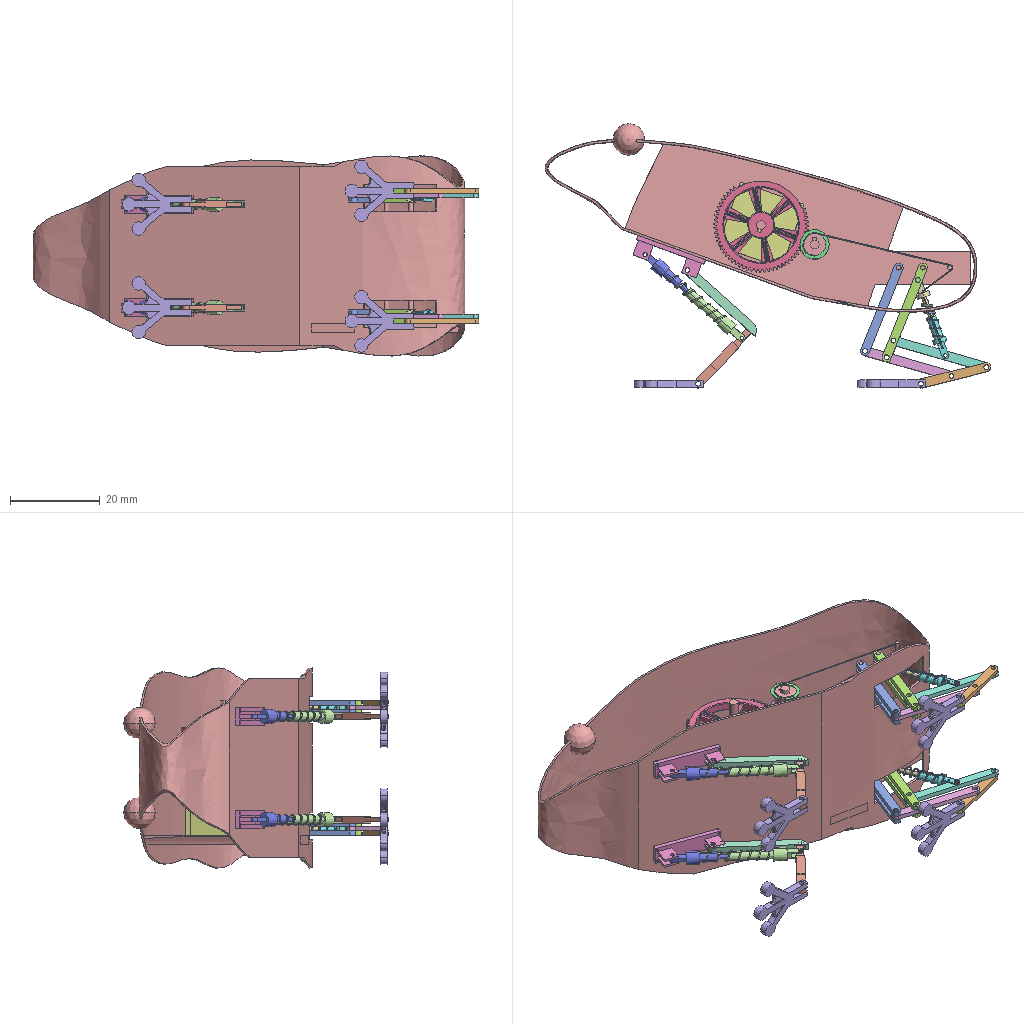Assembly | SolidWorks | 22 different items | 46 placed | box 99 x 59 x 45 mm
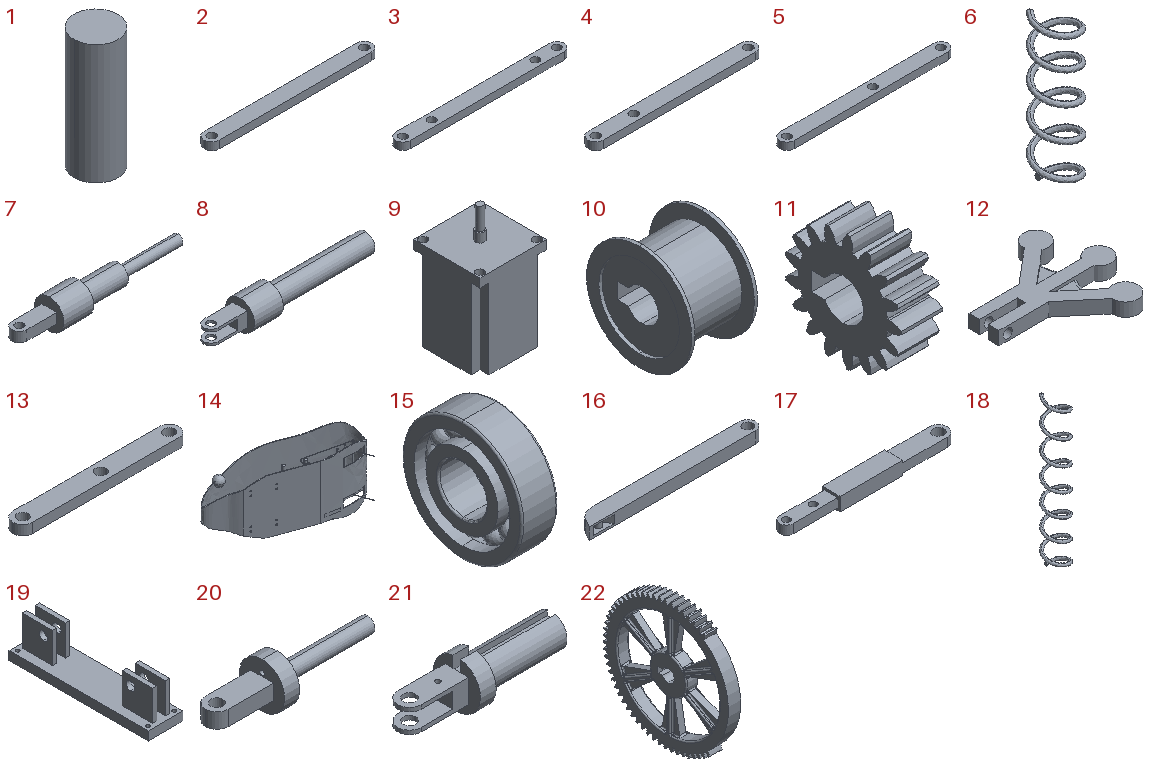Parts list (item | quantity | size | volume | features):
1 | x2 | 1.1 x 1.1 x 3 mm | 2.851 mm3 | features Extrusion 1
2 | x4 | 22 x 2 x 1 mm | 41.241 mm3 | features Extrusion 1, ICE 1
3 | x4 | 23.5 x 2 x 1 mm | 42.34 mm3 | features Extrusion 1, ICE 1
4 | x2 | 22 x 2 x 1 mm | 40.291 mm3 | features Extrusion 1, ICE 1
5 | x2 | 23.5 x 2 x 1 mm | 43.291 mm3 | features Extrusion 1, ICE 1
6 | x2 | 2.421 x 2.42 x 9.051 mm | 2.291 mm3 | features Helix 1, Sweep 1
7 | x2 | 16.75 x 3 x 3 mm | 43.365 mm3 | features ICE 2, Revolution 1
8 | x2 | 16.75 x 3 x 3 mm | 51.85 mm3 | features ICE 3, Revolution 1
9 | x1 | 15 x 15 x 27 mm | 4207 mm3 | features ICE 4, Extrusion 1
10 | x2 | 4.086 x 6.543 x 6.543 mm | 64.18 mm3 | features ICE 1, Revolution 1
11 | x1 | 2 x 5.664 x 5.687 mm | 31.821 mm3 | features BaseBody 1, ICE 1
12 | x4 | 15.281 x 13.766 x 1.6 mm | 106.552 mm3 | features ICE 7, Extrusion 1, Fillet 1, Scale 1
13 | x2 | 17 x 2 x 1 mm | 30.291 mm3 | features Extrusion 1, ICE 1
14 | x1 | 96.052 x 49.979 x 44.528 mm | 8210 mm3 | features ICE 13, MirrorPattern 3, Extrusion 1, Fillet 1, Revolution 1, Sweep 1
15 | x2 | 1.5 x 5 x 5 mm | 18.357 mm3 | features BaseBody 1
16 | x2 | 22.155 x 2 x 1.5 mm | 59.83 mm3 | features Extrusion 1, Fillet 1, ICE 1
17 | x2 | 18.75 x 2 x 1.5 mm | 38.722 mm3 | features ICE 2, Extrusion 1, MirrorPattern 1
18 | x2 | 2.421 x 2.421 x 16.049 mm | 3.23 mm3 | features Helix 1, Sweep 1
19 | x2 | 4 x 16 x 4.5 mm | 86.427 mm3 | features ICE 4, Extrusion 1
20 | x2 | 10.75 x 3 x 3 mm | 16.591 mm3 | features ICE 3, Revolution 1
21 | x2 | 9.75 x 3 x 2.979 mm | 20.717 mm3 | features ICE 5, Revolution 1
22 | x1 | 2 x 20.317 x 20.986 mm | 331.893 mm3 | features ICE 4, CirPattern 2, Fillet 2, BaseBody 1, MirrorPattern 1
Mates (type | each side: item.copy, entity, surface, feature):
Concentric | 14.1 face cylinder Boss-Extrude1 | 2.1 face cylinder Thigh1 length
Concentric | 14.1 face cylinder Boss-Extrude1 | 3.1 face cylinder Thigh1 length
Concentric | 2.1 face cylinder Thigh1 length | 4.1 face cylinder Thigh1 length
Concentric | 3.1 face cylinder Thigh1 length | 4.1 face cylinder Thigh1 length
Concentric | 3.1 face cylinder Thigh1 length | 5.1 face cylinder Thigh1 length
Coincident | 14.1 face plane Boss-Extrude1 | 3.1 face plane Thigh1 length
Coincident | 2.1 face plane Thigh1 length | 3.1 face plane Thigh1 length
Concentric | 4.1 face cylinder Thigh1 length | 13.1 face cylinder Thigh1 length
Concentric | 5.1 face cylinder Thigh1 length | 13.1 face cylinder Thigh1 length
Coincident | 3.1 face plane Thigh1 length | 5.1 face plane Thigh1 length
Coincident | 3.1 face plane Thigh1 length | 4.1 face plane Thigh1 length
Coincident | 3.1 face plane Thigh1 length | 13.1 face plane Thigh1 length
Lock | 13.1 select_type:0 | 12.1 select_type:0
Concentric | 2.1 face cylinder Thigh1 length | 2.2 face cylinder Thigh1 length
Concentric | 3.1 face cylinder Thigh1 length | 3.2 face cylinder Thigh1 length
Concentric | 4.1 face cylinder Thigh1 length | 3.2 face cylinder Thigh1 length
Concentric | 4.1 face cylinder Thigh1 length | 2.2 face cylinder Thigh1 length
Coincident | 5.1 face plane Thigh1 length | 3.2 face plane Thigh1 length
Coincident | 4.1 face plane Thigh1 length | 2.2 face plane Thigh1 length
Concentric | 3.1 face cylinder Thigh1 length | 1.1 face cylinder Boss-Extrude1
Coincident | 3.1 face plane Thigh1 length | 1.1 face plane Boss-Extrude1
Coincident | 22.1 face plane Input1 | 11.1 face plane Input1
Coincident | 14.1 face plane Boss-Extrude3 | 9.1 face plane Boss-Extrude1
Concentric | 14.1 face cylinder Boss-Extrude1 | 22.1 face cylinder Input1
Concentric | 14.1 face cylinder Boss-Extrude1 | 11.1 face cylinder Input1
Concentric | 14.1 face cylinder Boss-Extrude1 | 15.1 face cylinder Input1
Coincident | 14.1 face plane Cut-Extrude6 | 15.1 face plane Input1
Concentric | 14.1 face cylinder Boss-Extrude1 | 15.2 face cylinder Input1
Coincident | 14.1 face plane Cut-Extrude6 | 15.2 face plane Input1
Coincident | 14.1 face plane Boss-Extrude2 | 19.1 face plane Boss-Extrude1
Concentric | 14.1 face cylinder Cut-Extrude12 | 19.1 face cylinder Cut-Extrude2 | 2 times
Parallel | 16.1 face plane Cut-Extrude1 | 17.1 face plane Boss-Extrude3
Concentric | 16.1 face cylinder Cut-Extrude1 | 17.1 face cylinder Boss-Extrude3
Coincident | 16.1 face plane Cut-Extrude1 | 17.1 face plane Boss-Extrude3
Concentric | 17.1 edge | 8.1 edge
Coincident | 17.1 face plane Boss-Extrude3 | 8.1 face plane Cut-Extrude1
Coincident | 17.1 face plane Mirror1 | 12.2 face plane Boss-Extrude1
Concentric | 17.1 edge | 12.2 edge
Concentric | 7.1 edge | 8.1 edge
Parallel | 7.1 face plane Boss-Extrude1 | 8.1 face plane Boss-Extrude1
Concentric | 7.1 face cylinder Boss-Extrude1 | 19.1 face cylinder Cut-Extrude1 | 2 times
Coincident | 7.1 face plane Boss-Extrude1 | 19.1 face plane Boss-Extrude2
Concentric | 16.1 face cylinder Boss-Extrude2 | 19.1 face cylinder Cut-Extrude1
Concentric | 5.1 face cylinder Thigh1 length | 21.1 face cylinder Boss-Extrude1
Coincident | 5.1 face plane Thigh1 length | 21.1 face plane Cut-Extrude1
Concentric | 1.1 face cylinder Boss-Extrude1 | 20.1 face cylinder Boss-Extrude1
Coincident | 3.1 face plane Thigh1 length | 20.1 face plane Boss-Extrude1
Concentric | 21.1 face cylinder Revolve1 | 20.1 face cylinder Cut-Extrude3
Concentric | 14.1 face cylinder Boss-Extrude1 | 10.1 face cylinder Revolve1
DistanceDim | 14.1 face plane Boss-Extrude1 | 10.1 face plane Revolve1
Concentric | 21.1 face cylinder Revolve1 | 6.1 select_type:24
Coincident | 21.2 face cylinder Revolve1 | 6.2 select_type:24
Coincident | 21.2 face plane Revolve1 | 6.2 select_type:24
Coincident | 21.1 face plane Revolve1 | 6.1 select_type:24
Coincident | 8.1 face cylinder Revolve1 | 18.1 select_type:24
Coincident | 8.1 face plane Revolve1 | 18.1 select_type:24
Coincident | 8.2 face cylinder Revolve1 | 18.2 select_type:24
Coincident | 8.2 face plane Revolve1 | 18.2 select_type:24
DistanceDim | 22.1 face plane Input1 | 9.1 face plane Boss-Extrude1
Lock | 14.1 select_type:0 | 9.1 select_type:0